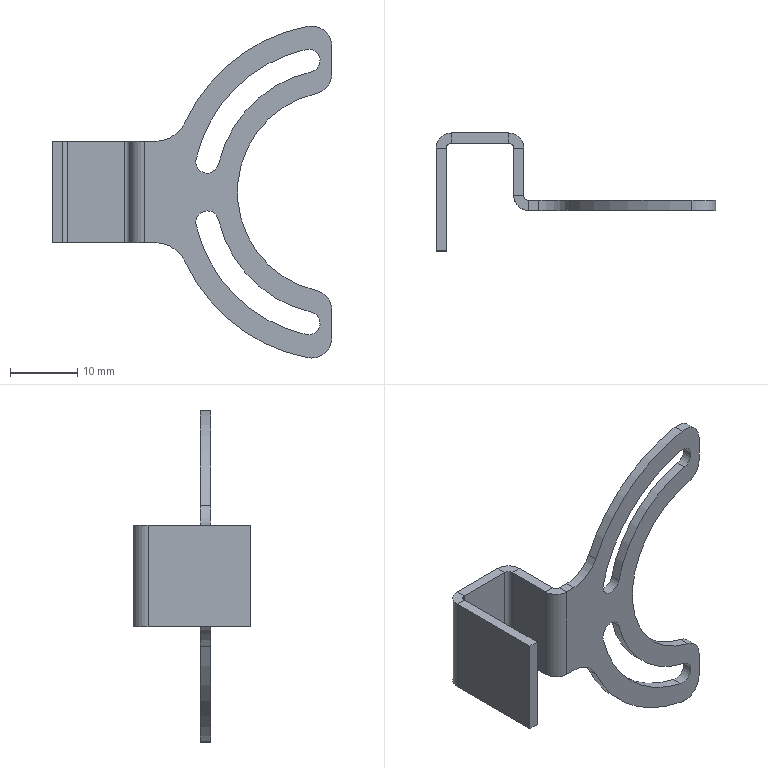Part | NX | features BREP 1 | 1 solid | 51 faces | box 41.5 x 17.5 x 49.267 mm | volume 1595 mm3 | cylinder 26 | plane 25 | commonest cylinder face diameters 3.4 x6 6 x5 1.473 x3 4.473 x3 10 x2 36.6 x2
STEP:
#1=CARTESIAN_POINT('',(27.,1.5,-24.633));
#2=VERTEX_POINT('',#1);
#3=CARTESIAN_POINT('',(26.455,1.5,-24.583));
#4=VERTEX_POINT('',#3);
#5=CARTESIAN_POINT('',(27.,1.5,-21.633));
#6=DIRECTION('',(0.,1.,0.));
#7=DIRECTION('',(0.,0.,-1.));
#8=AXIS2_PLACEMENT_3D('',#5,#6,#7);
#9=CIRCLE('',#8,3.);
#10=EDGE_CURVE('',#2,#4,#9,.T.);
#11=ORIENTED_EDGE('',*,*,#10,.F.);
#12=CARTESIAN_POINT('',(27.,0.,-24.633));
#13=VERTEX_POINT('',#12);
#14=CARTESIAN_POINT('',(27.,0.,-24.633));
#15=DIRECTION('',(0.,-1.,0.));
#16=VECTOR('',#15,1000.);
#17=LINE('',#14,#16);
#18=EDGE_CURVE('',#2,#13,#17,.T.);
#19=ORIENTED_EDGE('',*,*,#18,.T.);
#20=CARTESIAN_POINT('',(26.455,0.,-24.583));
#21=VERTEX_POINT('',#20);
#22=CARTESIAN_POINT('',(27.,0.,-21.633));
#23=DIRECTION('',(0.,-1.,0.));
#24=DIRECTION('',(0.,0.,-1.));
#25=AXIS2_PLACEMENT_3D('',#22,#23,#24);
#26=CIRCLE('',#25,3.);
#27=EDGE_CURVE('',#21,#13,#26,.T.);
#28=ORIENTED_EDGE('',*,*,#27,.F.);
#29=CARTESIAN_POINT('',(26.455,0.,-24.583));
#30=DIRECTION('',(0.,-1.,0.));
#31=VECTOR('',#30,1000.);
#32=LINE('',#29,#31);
#33=EDGE_CURVE('',#4,#21,#32,.T.);
#34=ORIENTED_EDGE('',*,*,#33,.F.);
#35=EDGE_LOOP('',(#11,#19,#28,#34));
#36=FACE_BOUND('',#35,.T.);
#37=CARTESIAN_POINT('',(27.,0.,-21.633));
#38=DIRECTION('',(0.,-1.,0.));
#39=DIRECTION('',(0.,0.,1.));
#40=AXIS2_PLACEMENT_3D('',#37,#38,#39);
#41=CYLINDRICAL_SURFACE('',#40,3.);
#42=ADVANCED_FACE('',(#36),#41,.T.);
#43=CARTESIAN_POINT('',(26.934,0.,17.843));
#44=VERTEX_POINT('',#43);
#45=CARTESIAN_POINT('',(26.556,0.,21.2));
#46=VERTEX_POINT('',#45);
#47=CARTESIAN_POINT('',(26.556,0.,19.5));
#48=DIRECTION('',(0.,-1.,0.));
#49=DIRECTION('',(0.,0.,-1.));
#50=AXIS2_PLACEMENT_3D('',#47,#48,#49);
#51=CIRCLE('',#50,1.7);
#52=EDGE_CURVE('',#44,#46,#51,.T.);
#53=ORIENTED_EDGE('',*,*,#52,.T.);
#54=CARTESIAN_POINT('',(26.556,1.5,21.2));
#55=VERTEX_POINT('',#54);
#56=CARTESIAN_POINT('',(26.556,-6.,21.2));
#57=DIRECTION('',(0.,1.,0.));
#58=VECTOR('',#57,1000.);
#59=LINE('',#56,#58);
#60=EDGE_CURVE('',#46,#55,#59,.T.);
#61=ORIENTED_EDGE('',*,*,#60,.T.);
#62=CARTESIAN_POINT('',(26.934,1.5,17.843));
#63=VERTEX_POINT('',#62);
#64=CARTESIAN_POINT('',(26.556,1.5,19.5));
#65=DIRECTION('',(0.,-1.,0.));
#66=DIRECTION('',(0.,0.,-1.));
#67=AXIS2_PLACEMENT_3D('',#64,#65,#66);
#68=CIRCLE('',#67,1.7);
#69=EDGE_CURVE('',#63,#55,#68,.T.);
#70=ORIENTED_EDGE('',*,*,#69,.F.);
#71=CARTESIAN_POINT('',(26.934,-6.,17.843));
#72=DIRECTION('',(0.,1.,0.));
#73=VECTOR('',#72,1000.);
#74=LINE('',#71,#73);
#75=EDGE_CURVE('',#44,#63,#74,.T.);
#76=ORIENTED_EDGE('',*,*,#75,.F.);
#77=EDGE_LOOP('',(#53,#61,#70,#76));
#78=FACE_BOUND('',#77,.T.);
#79=CARTESIAN_POINT('',(26.556,-6.,19.5));
#80=DIRECTION('',(0.,1.,0.));
#81=DIRECTION('',(0.,0.,-1.));
#82=AXIS2_PLACEMENT_3D('',#79,#80,#81);
#83=CYLINDRICAL_SURFACE('',#82,1.7);
#84=ADVANCED_FACE('',(#78),#83,.F.);
#85=CARTESIAN_POINT('',(13.169,0.,-4.117));
#86=VERTEX_POINT('',#85);
#87=CARTESIAN_POINT('',(11.513,0.,-2.8));
#88=VERTEX_POINT('',#87);
#89=CARTESIAN_POINT('',(11.513,0.,-4.5));
#90=DIRECTION('',(0.,-1.,0.));
#91=DIRECTION('',(0.,0.,-1.));
#92=AXIS2_PLACEMENT_3D('',#89,#90,#91);
#93=CIRCLE('',#92,1.7);
#94=EDGE_CURVE('',#86,#88,#93,.T.);
#95=ORIENTED_EDGE('',*,*,#94,.T.);
#96=CARTESIAN_POINT('',(11.513,1.5,-2.8));
#97=VERTEX_POINT('',#96);
#98=CARTESIAN_POINT('',(11.513,-6.,-2.8));
#99=DIRECTION('',(0.,1.,0.));
#100=VECTOR('',#99,1000.);
#101=LINE('',#98,#100);
#102=EDGE_CURVE('',#88,#97,#101,.T.);
#103=ORIENTED_EDGE('',*,*,#102,.T.);
#104=CARTESIAN_POINT('',(13.169,1.5,-4.117));
#105=VERTEX_POINT('',#104);
#106=CARTESIAN_POINT('',(11.513,1.5,-4.5));
#107=DIRECTION('',(0.,-1.,0.));
#108=DIRECTION('',(0.,0.,-1.));
#109=AXIS2_PLACEMENT_3D('',#106,#107,#108);
#110=CIRCLE('',#109,1.7);
#111=EDGE_CURVE('',#105,#97,#110,.T.);
#112=ORIENTED_EDGE('',*,*,#111,.F.);
#113=CARTESIAN_POINT('',(13.169,-6.,-4.117));
#114=DIRECTION('',(0.,1.,0.));
#115=VECTOR('',#114,1000.);
#116=LINE('',#113,#115);
#117=EDGE_CURVE('',#86,#105,#116,.T.);
#118=ORIENTED_EDGE('',*,*,#117,.F.);
#119=EDGE_LOOP('',(#95,#103,#112,#118));
#120=FACE_BOUND('',#119,.T.);
#121=CARTESIAN_POINT('',(11.513,-6.,-4.5));
#122=DIRECTION('',(0.,1.,0.));
#123=DIRECTION('',(0.,0.,-1.));
#124=AXIS2_PLACEMENT_3D('',#121,#122,#123);
#125=CYLINDRICAL_SURFACE('',#124,1.7);
#126=ADVANCED_FACE('',(#120),#125,.F.);
#127=CARTESIAN_POINT('',(26.178,0.,-21.157));
#128=VERTEX_POINT('',#127);
#129=CARTESIAN_POINT('',(26.934,0.,-17.843));
#130=VERTEX_POINT('',#129);
#131=CARTESIAN_POINT('',(26.556,0.,-19.5));
#132=DIRECTION('',(0.,-1.,0.));
#133=DIRECTION('',(0.,0.,-1.));
#134=AXIS2_PLACEMENT_3D('',#131,#132,#133);
#135=CIRCLE('',#134,1.7);
#136=EDGE_CURVE('',#128,#130,#135,.T.);
#137=ORIENTED_EDGE('',*,*,#136,.F.);
#138=CARTESIAN_POINT('',(9.856,0.,-4.883));
#139=VERTEX_POINT('',#138);
#140=CARTESIAN_POINT('',(31.,0.,0.));
#141=DIRECTION('',(0.,-1.,0.));
#142=DIRECTION('',(0.,0.,-1.));
#143=AXIS2_PLACEMENT_3D('',#140,#141,#142);
#144=CIRCLE('',#143,21.7);
#145=EDGE_CURVE('',#139,#128,#144,.T.);
#146=ORIENTED_EDGE('',*,*,#145,.F.);
#147=CARTESIAN_POINT('',(11.513,0.,-4.5));
#148=DIRECTION('',(0.,-1.,0.));
#149=DIRECTION('',(0.,0.,-1.));
#150=AXIS2_PLACEMENT_3D('',#147,#148,#149);
#151=CIRCLE('',#150,1.7);
#152=EDGE_CURVE('',#88,#139,#151,.T.);
#153=ORIENTED_EDGE('',*,*,#152,.F.);
#154=ORIENTED_EDGE('',*,*,#94,.F.);
#155=CARTESIAN_POINT('',(31.,0.,0.));
#156=DIRECTION('',(0.,1.,0.));
#157=DIRECTION('',(0.,0.,-1.));
#158=AXIS2_PLACEMENT_3D('',#155,#156,#157);
#159=CIRCLE('',#158,18.3);
#160=EDGE_CURVE('',#130,#86,#159,.T.);
#161=ORIENTED_EDGE('',*,*,#160,.F.);
#162=EDGE_LOOP('',(#137,#146,#153,#154,#161));
#163=FACE_BOUND('',#162,.T.);
#164=ORIENTED_EDGE('',*,*,#52,.F.);
#165=CARTESIAN_POINT('',(13.169,0.,4.117));
#166=VERTEX_POINT('',#165);
#167=CARTESIAN_POINT('',(31.,0.,0.));
#168=DIRECTION('',(0.,1.,0.));
#169=DIRECTION('',(0.,0.,-1.));
#170=AXIS2_PLACEMENT_3D('',#167,#168,#169);
#171=CIRCLE('',#170,18.3);
#172=EDGE_CURVE('',#166,#44,#171,.T.);
#173=ORIENTED_EDGE('',*,*,#172,.F.);
#174=CARTESIAN_POINT('',(9.856,0.,4.883));
#175=VERTEX_POINT('',#174);
#176=CARTESIAN_POINT('',(11.513,0.,4.5));
#177=DIRECTION('',(0.,-1.,0.));
#178=DIRECTION('',(0.,0.,-1.));
#179=AXIS2_PLACEMENT_3D('',#176,#177,#178);
#180=CIRCLE('',#179,1.7);
#181=EDGE_CURVE('',#175,#166,#180,.T.);
#182=ORIENTED_EDGE('',*,*,#181,.F.);
#183=CARTESIAN_POINT('',(26.178,0.,21.157));
#184=VERTEX_POINT('',#183);
#185=CARTESIAN_POINT('',(31.,0.,0.));
#186=DIRECTION('',(0.,-1.,0.));
#187=DIRECTION('',(0.,0.,-1.));
#188=AXIS2_PLACEMENT_3D('',#185,#186,#187);
#189=CIRCLE('',#188,21.7);
#190=EDGE_CURVE('',#184,#175,#189,.T.);
#191=ORIENTED_EDGE('',*,*,#190,.F.);
#192=CARTESIAN_POINT('',(26.556,0.,19.5));
#193=DIRECTION('',(0.,-1.,0.));
#194=DIRECTION('',(0.,0.,-1.));
#195=AXIS2_PLACEMENT_3D('',#192,#193,#194);
#196=CIRCLE('',#195,1.7);
#197=EDGE_CURVE('',#46,#184,#196,.T.);
#198=ORIENTED_EDGE('',*,*,#197,.F.);
#199=EDGE_LOOP('',(#164,#173,#182,#191,#198));
#200=FACE_BOUND('',#199,.T.);
#201=CARTESIAN_POINT('',(8.274,0.,-10.417));
#202=VERTEX_POINT('',#201);
#203=CARTESIAN_POINT('',(31.,0.,0.));
#204=DIRECTION('',(0.,1.,0.));
#205=DIRECTION('',(0.,0.,-1.));
#206=AXIS2_PLACEMENT_3D('',#203,#204,#205);
#207=CIRCLE('',#206,25.);
#208=EDGE_CURVE('',#21,#202,#207,.T.);
#209=ORIENTED_EDGE('',*,*,#208,.F.);
#210=ORIENTED_EDGE('',*,*,#27,.T.);
#211=CARTESIAN_POINT('',(30.,0.,-21.633));
#212=VERTEX_POINT('',#211);
#213=CARTESIAN_POINT('',(27.,0.,-21.633));
#214=DIRECTION('',(0.,-1.,0.));
#215=DIRECTION('',(0.,0.,-1.));
#216=AXIS2_PLACEMENT_3D('',#213,#214,#215);
#217=CIRCLE('',#216,3.);
#218=EDGE_CURVE('',#13,#212,#217,.T.);
#219=ORIENTED_EDGE('',*,*,#218,.T.);
#220=CARTESIAN_POINT('',(30.,0.,-17.55));
#221=VERTEX_POINT('',#220);
#222=CARTESIAN_POINT('',(30.,0.,25.));
#223=DIRECTION('',(0.,0.,-1.));
#224=VECTOR('',#223,1000.);
#225=LINE('',#222,#224);
#226=EDGE_CURVE('',#221,#212,#225,.T.);
#227=ORIENTED_EDGE('',*,*,#226,.F.);
#228=CARTESIAN_POINT('',(27.667,0.,-14.625));
#229=VERTEX_POINT('',#228);
#230=CARTESIAN_POINT('',(27.,0.,-17.55));
#231=DIRECTION('',(0.,-1.,0.));
#232=DIRECTION('',(0.,0.,-1.));
#233=AXIS2_PLACEMENT_3D('',#230,#231,#232);
#234=CIRCLE('',#233,3.);
#235=EDGE_CURVE('',#221,#229,#234,.T.);
#236=ORIENTED_EDGE('',*,*,#235,.T.);
#237=CARTESIAN_POINT('',(27.667,0.,14.625));
#238=VERTEX_POINT('',#237);
#239=CARTESIAN_POINT('',(31.,0.,0.));
#240=DIRECTION('',(0.,-1.,0.));
#241=DIRECTION('',(0.,0.,-1.));
#242=AXIS2_PLACEMENT_3D('',#239,#240,#241);
#243=CIRCLE('',#242,15.);
#244=EDGE_CURVE('',#238,#229,#243,.T.);
#245=ORIENTED_EDGE('',*,*,#244,.F.);
#246=CARTESIAN_POINT('',(30.,0.,17.55));
#247=VERTEX_POINT('',#246);
#248=CARTESIAN_POINT('',(27.,0.,17.55));
#249=DIRECTION('',(0.,-1.,0.));
#250=DIRECTION('',(0.,0.,-1.));
#251=AXIS2_PLACEMENT_3D('',#248,#249,#250);
#252=CIRCLE('',#251,3.);
#253=EDGE_CURVE('',#238,#247,#252,.T.);
#254=ORIENTED_EDGE('',*,*,#253,.T.);
#255=CARTESIAN_POINT('',(30.,0.,21.633));
#256=VERTEX_POINT('',#255);
#257=CARTESIAN_POINT('',(30.,0.,25.));
#258=DIRECTION('',(0.,0.,-1.));
#259=VECTOR('',#258,1000.);
#260=LINE('',#257,#259);
#261=EDGE_CURVE('',#256,#247,#260,.T.);
#262=ORIENTED_EDGE('',*,*,#261,.F.);
#263=CARTESIAN_POINT('',(26.455,0.,24.583));
#264=VERTEX_POINT('',#263);
#265=CARTESIAN_POINT('',(27.,0.,21.633));
#266=DIRECTION('',(0.,-1.,0.));
#267=DIRECTION('',(0.,0.,-1.));
#268=AXIS2_PLACEMENT_3D('',#265,#266,#267);
#269=CIRCLE('',#268,3.);
#270=EDGE_CURVE('',#256,#264,#269,.T.);
#271=ORIENTED_EDGE('',*,*,#270,.T.);
#272=CARTESIAN_POINT('',(8.274,0.,10.417));
#273=VERTEX_POINT('',#272);
#274=CARTESIAN_POINT('',(31.,0.,0.));
#275=DIRECTION('',(0.,1.,0.));
#276=DIRECTION('',(0.,0.,-1.));
#277=AXIS2_PLACEMENT_3D('',#274,#275,#276);
#278=CIRCLE('',#277,25.);
#279=EDGE_CURVE('',#273,#264,#278,.T.);
#280=ORIENTED_EDGE('',*,*,#279,.F.);
#281=CARTESIAN_POINT('',(3.728,0.,7.5));
#282=VERTEX_POINT('',#281);
#283=CARTESIAN_POINT('',(3.728,0.,12.5));
#284=DIRECTION('',(0.,1.,0.));
#285=DIRECTION('',(0.,0.,-1.));
#286=AXIS2_PLACEMENT_3D('',#283,#284,#285);
#287=CIRCLE('',#286,5.);
#288=EDGE_CURVE('',#273,#282,#287,.T.);
#289=ORIENTED_EDGE('',*,*,#288,.T.);
#290=CARTESIAN_POINT('',(2.237,0.,7.5));
#291=VERTEX_POINT('',#290);
#292=CARTESIAN_POINT('',(0.,0.,7.5));
#293=DIRECTION('',(1.,0.,0.));
#294=VECTOR('',#293,1000.);
#295=LINE('',#292,#294);
#296=EDGE_CURVE('',#291,#282,#295,.T.);
#297=ORIENTED_EDGE('',*,*,#296,.F.);
#298=CARTESIAN_POINT('',(2.237,0.,-7.5));
#299=VERTEX_POINT('',#298);
#300=CARTESIAN_POINT('',(2.237,0.,25.));
#301=DIRECTION('',(0.,0.,-1.));
#302=VECTOR('',#301,1000.);
#303=LINE('',#300,#302);
#304=EDGE_CURVE('',#291,#299,#303,.T.);
#305=ORIENTED_EDGE('',*,*,#304,.T.);
#306=CARTESIAN_POINT('',(3.728,0.,-7.5));
#307=VERTEX_POINT('',#306);
#308=CARTESIAN_POINT('',(0.,0.,-7.5));
#309=DIRECTION('',(-1.,0.,0.));
#310=VECTOR('',#309,1000.);
#311=LINE('',#308,#310);
#312=EDGE_CURVE('',#307,#299,#311,.T.);
#313=ORIENTED_EDGE('',*,*,#312,.F.);
#314=CARTESIAN_POINT('',(3.728,0.,-12.5));
#315=DIRECTION('',(0.,1.,0.));
#316=DIRECTION('',(0.,0.,-1.));
#317=AXIS2_PLACEMENT_3D('',#314,#315,#316);
#318=CIRCLE('',#317,5.);
#319=EDGE_CURVE('',#307,#202,#318,.T.);
#320=ORIENTED_EDGE('',*,*,#319,.T.);
#321=EDGE_LOOP('',(#209,#210,#219,#227,#236,#245,#254,#262,#271,#280,#289,#297,#305,#313,#320));
#322=FACE_BOUND('',#321,.T.);
#323=CARTESIAN_POINT('',(0.,0.,25.));
#324=DIRECTION('',(0.,-1.,0.));
#325=DIRECTION('',(0.,0.,1.));
#326=AXIS2_PLACEMENT_3D('',#323,#324,#325);
#327=PLANE('',#326);
#328=ADVANCED_FACE('',(#163,#200,#322),#327,.T.);
#329=CARTESIAN_POINT('',(9.856,1.5,-4.883));
#330=VERTEX_POINT('',#329);
#331=CARTESIAN_POINT('',(26.178,1.5,-21.157));
#332=VERTEX_POINT('',#331);
#333=CARTESIAN_POINT('',(31.,1.5,0.));
#334=DIRECTION('',(0.,-1.,0.));
#335=DIRECTION('',(0.,0.,-1.));
#336=AXIS2_PLACEMENT_3D('',#333,#334,#335);
#337=CIRCLE('',#336,21.7);
#338=EDGE_CURVE('',#330,#332,#337,.T.);
#339=ORIENTED_EDGE('',*,*,#338,.T.);
#340=CARTESIAN_POINT('',(26.934,1.5,-17.843));
#341=VERTEX_POINT('',#340);
#342=CARTESIAN_POINT('',(26.556,1.5,-19.5));
#343=DIRECTION('',(0.,-1.,0.));
#344=DIRECTION('',(0.,0.,-1.));
#345=AXIS2_PLACEMENT_3D('',#342,#343,#344);
#346=CIRCLE('',#345,1.7);
#347=EDGE_CURVE('',#332,#341,#346,.T.);
#348=ORIENTED_EDGE('',*,*,#347,.T.);
#349=CARTESIAN_POINT('',(31.,1.5,0.));
#350=DIRECTION('',(0.,1.,0.));
#351=DIRECTION('',(0.,0.,-1.));
#352=AXIS2_PLACEMENT_3D('',#349,#350,#351);
#353=CIRCLE('',#352,18.3);
#354=EDGE_CURVE('',#341,#105,#353,.T.);
#355=ORIENTED_EDGE('',*,*,#354,.T.);
#356=ORIENTED_EDGE('',*,*,#111,.T.);
#357=CARTESIAN_POINT('',(11.513,1.5,-4.5));
#358=DIRECTION('',(0.,-1.,0.));
#359=DIRECTION('',(0.,0.,-1.));
#360=AXIS2_PLACEMENT_3D('',#357,#358,#359);
#361=CIRCLE('',#360,1.7);
#362=EDGE_CURVE('',#97,#330,#361,.T.);
#363=ORIENTED_EDGE('',*,*,#362,.T.);
#364=EDGE_LOOP('',(#339,#348,#355,#356,#363));
#365=FACE_BOUND('',#364,.T.);
#366=CARTESIAN_POINT('',(13.169,1.5,4.117));
#367=VERTEX_POINT('',#366);
#368=CARTESIAN_POINT('',(31.,1.5,0.));
#369=DIRECTION('',(0.,1.,0.));
#370=DIRECTION('',(0.,0.,-1.));
#371=AXIS2_PLACEMENT_3D('',#368,#369,#370);
#372=CIRCLE('',#371,18.3);
#373=EDGE_CURVE('',#367,#63,#372,.T.);
#374=ORIENTED_EDGE('',*,*,#373,.T.);
#375=ORIENTED_EDGE('',*,*,#69,.T.);
#376=CARTESIAN_POINT('',(26.178,1.5,21.157));
#377=VERTEX_POINT('',#376);
#378=CARTESIAN_POINT('',(26.556,1.5,19.5));
#379=DIRECTION('',(0.,-1.,0.));
#380=DIRECTION('',(0.,0.,-1.));
#381=AXIS2_PLACEMENT_3D('',#378,#379,#380);
#382=CIRCLE('',#381,1.7);
#383=EDGE_CURVE('',#55,#377,#382,.T.);
#384=ORIENTED_EDGE('',*,*,#383,.T.);
#385=CARTESIAN_POINT('',(9.856,1.5,4.883));
#386=VERTEX_POINT('',#385);
#387=CARTESIAN_POINT('',(31.,1.5,0.));
#388=DIRECTION('',(0.,-1.,0.));
#389=DIRECTION('',(0.,0.,-1.));
#390=AXIS2_PLACEMENT_3D('',#387,#388,#389);
#391=CIRCLE('',#390,21.7);
#392=EDGE_CURVE('',#377,#386,#391,.T.);
#393=ORIENTED_EDGE('',*,*,#392,.T.);
#394=CARTESIAN_POINT('',(11.513,1.5,4.5));
#395=DIRECTION('',(0.,-1.,0.));
#396=DIRECTION('',(0.,0.,-1.));
#397=AXIS2_PLACEMENT_3D('',#394,#395,#396);
#398=CIRCLE('',#397,1.7);
#399=EDGE_CURVE('',#386,#367,#398,.T.);
#400=ORIENTED_EDGE('',*,*,#399,.T.);
#401=EDGE_LOOP('',(#374,#375,#384,#393,#400));
#402=FACE_BOUND('',#401,.T.);
#403=CARTESIAN_POINT('',(30.,1.5,-17.55));
#404=VERTEX_POINT('',#403);
#405=CARTESIAN_POINT('',(30.,1.5,-21.633));
#406=VERTEX_POINT('',#405);
#407=CARTESIAN_POINT('',(30.,1.5,25.));
#408=DIRECTION('',(0.,0.,-1.));
#409=VECTOR('',#408,1000.);
#410=LINE('',#407,#409);
#411=EDGE_CURVE('',#404,#406,#410,.T.);
#412=ORIENTED_EDGE('',*,*,#411,.T.);
#413=CARTESIAN_POINT('',(27.,1.5,-21.633));
#414=DIRECTION('',(0.,1.,0.));
#415=DIRECTION('',(0.,0.,-1.));
#416=AXIS2_PLACEMENT_3D('',#413,#414,#415);
#417=CIRCLE('',#416,3.);
#418=EDGE_CURVE('',#406,#2,#417,.T.);
#419=ORIENTED_EDGE('',*,*,#418,.T.);
#420=ORIENTED_EDGE('',*,*,#10,.T.);
#421=CARTESIAN_POINT('',(8.274,1.5,-10.417));
#422=VERTEX_POINT('',#421);
#423=CARTESIAN_POINT('',(31.,1.5,0.));
#424=DIRECTION('',(0.,1.,0.));
#425=DIRECTION('',(0.,0.,-1.));
#426=AXIS2_PLACEMENT_3D('',#423,#424,#425);
#427=CIRCLE('',#426,25.);
#428=EDGE_CURVE('',#4,#422,#427,.T.);
#429=ORIENTED_EDGE('',*,*,#428,.T.);
#430=CARTESIAN_POINT('',(3.728,1.5,-7.5));
#431=VERTEX_POINT('',#430);
#432=CARTESIAN_POINT('',(3.728,1.5,-12.5));
#433=DIRECTION('',(0.,-1.,0.));
#434=DIRECTION('',(0.,0.,-1.));
#435=AXIS2_PLACEMENT_3D('',#432,#433,#434);
#436=CIRCLE('',#435,5.);
#437=EDGE_CURVE('',#422,#431,#436,.T.);
#438=ORIENTED_EDGE('',*,*,#437,.T.);
#439=CARTESIAN_POINT('',(2.237,1.5,-7.5));
#440=VERTEX_POINT('',#439);
#441=CARTESIAN_POINT('',(0.,1.5,-7.5));
#442=DIRECTION('',(-1.,0.,0.));
#443=VECTOR('',#442,1000.);
#444=LINE('',#441,#443);
#445=EDGE_CURVE('',#431,#440,#444,.T.);
#446=ORIENTED_EDGE('',*,*,#445,.T.);
#447=CARTESIAN_POINT('',(2.237,1.5,7.5));
#448=VERTEX_POINT('',#447);
#449=CARTESIAN_POINT('',(2.237,1.5,25.));
#450=DIRECTION('',(0.,0.,-1.));
#451=VECTOR('',#450,1000.);
#452=LINE('',#449,#451);
#453=EDGE_CURVE('',#448,#440,#452,.T.);
#454=ORIENTED_EDGE('',*,*,#453,.F.);
#455=CARTESIAN_POINT('',(3.728,1.5,7.5));
#456=VERTEX_POINT('',#455);
#457=CARTESIAN_POINT('',(0.,1.5,7.5));
#458=DIRECTION('',(1.,0.,0.));
#459=VECTOR('',#458,1000.);
#460=LINE('',#457,#459);
#461=EDGE_CURVE('',#448,#456,#460,.T.);
#462=ORIENTED_EDGE('',*,*,#461,.T.);
#463=CARTESIAN_POINT('',(8.274,1.5,10.417));
#464=VERTEX_POINT('',#463);
#465=CARTESIAN_POINT('',(3.728,1.5,12.5));
#466=DIRECTION('',(0.,-1.,0.));
#467=DIRECTION('',(0.,0.,-1.));
#468=AXIS2_PLACEMENT_3D('',#465,#466,#467);
#469=CIRCLE('',#468,5.);
#470=EDGE_CURVE('',#456,#464,#469,.T.);
#471=ORIENTED_EDGE('',*,*,#470,.T.);
#472=CARTESIAN_POINT('',(26.455,1.5,24.583));
#473=VERTEX_POINT('',#472);
#474=CARTESIAN_POINT('',(31.,1.5,0.));
#475=DIRECTION('',(0.,1.,0.));
#476=DIRECTION('',(0.,0.,-1.));
#477=AXIS2_PLACEMENT_3D('',#474,#475,#476);
#478=CIRCLE('',#477,25.);
#479=EDGE_CURVE('',#464,#473,#478,.T.);
#480=ORIENTED_EDGE('',*,*,#479,.T.);
#481=CARTESIAN_POINT('',(30.,1.5,21.633));
#482=VERTEX_POINT('',#481);
#483=CARTESIAN_POINT('',(27.,1.5,21.633));
#484=DIRECTION('',(0.,1.,0.));
#485=DIRECTION('',(0.,0.,-1.));
#486=AXIS2_PLACEMENT_3D('',#483,#484,#485);
#487=CIRCLE('',#486,3.);
#488=EDGE_CURVE('',#473,#482,#487,.T.);
#489=ORIENTED_EDGE('',*,*,#488,.T.);
#490=CARTESIAN_POINT('',(30.,1.5,17.55));
#491=VERTEX_POINT('',#490);
#492=CARTESIAN_POINT('',(30.,1.5,25.));
#493=DIRECTION('',(0.,0.,-1.));
#494=VECTOR('',#493,1000.);
#495=LINE('',#492,#494);
#496=EDGE_CURVE('',#482,#491,#495,.T.);
#497=ORIENTED_EDGE('',*,*,#496,.T.);
#498=CARTESIAN_POINT('',(27.667,1.5,14.625));
#499=VERTEX_POINT('',#498);
#500=CARTESIAN_POINT('',(27.,1.5,17.55));
#501=DIRECTION('',(0.,1.,0.));
#502=DIRECTION('',(0.,0.,-1.));
#503=AXIS2_PLACEMENT_3D('',#500,#501,#502);
#504=CIRCLE('',#503,3.);
#505=EDGE_CURVE('',#491,#499,#504,.T.);
#506=ORIENTED_EDGE('',*,*,#505,.T.);
#507=CARTESIAN_POINT('',(27.667,1.5,-14.625));
#508=VERTEX_POINT('',#507);
#509=CARTESIAN_POINT('',(31.,1.5,0.));
#510=DIRECTION('',(0.,-1.,0.));
#511=DIRECTION('',(0.,0.,-1.));
#512=AXIS2_PLACEMENT_3D('',#509,#510,#511);
#513=CIRCLE('',#512,15.);
#514=EDGE_CURVE('',#499,#508,#513,.T.);
#515=ORIENTED_EDGE('',*,*,#514,.T.);
#516=CARTESIAN_POINT('',(27.,1.5,-17.55));
#517=DIRECTION('',(0.,1.,0.));
#518=DIRECTION('',(0.,0.,-1.));
#519=AXIS2_PLACEMENT_3D('',#516,#517,#518);
#520=CIRCLE('',#519,3.);
#521=EDGE_CURVE('',#508,#404,#520,.T.);
#522=ORIENTED_EDGE('',*,*,#521,.T.);
#523=EDGE_LOOP('',(#412,#419,#420,#429,#438,#446,#454,#462,#471,#480,#489,#497,#506,#515,#522));
#524=FACE_BOUND('',#523,.T.);
#525=CARTESIAN_POINT('',(0.,1.5,25.));
#526=DIRECTION('',(0.,-1.,0.));
#527=DIRECTION('',(0.,0.,1.));
#528=AXIS2_PLACEMENT_3D('',#525,#526,#527);
#529=PLANE('',#528);
#530=ADVANCED_FACE('',(#365,#402,#524),#529,.F.);
#531=CARTESIAN_POINT('',(-11.5,-6.,-7.5));
#532=VERTEX_POINT('',#531);
#533=CARTESIAN_POINT('',(-11.5,9.263,-7.5));
#534=VERTEX_POINT('',#533);
#535=CARTESIAN_POINT('',(-11.5,-6.,-7.5));
#536=DIRECTION('',(0.,1.,0.));
#537=VECTOR('',#536,1000.);
#538=LINE('',#535,#537);
#539=EDGE_CURVE('',#532,#534,#538,.T.);
#540=ORIENTED_EDGE('',*,*,#539,.F.);
#541=CARTESIAN_POINT('',(-11.5,-6.,7.5));
#542=VERTEX_POINT('',#541);
#543=CARTESIAN_POINT('',(-11.5,-6.,25.));
#544=DIRECTION('',(0.,0.,-1.));
#545=VECTOR('',#544,1000.);
#546=LINE('',#543,#545);
#547=EDGE_CURVE('',#542,#532,#546,.T.);
#548=ORIENTED_EDGE('',*,*,#547,.F.);
#549=CARTESIAN_POINT('',(-11.5,9.263,7.5));
#550=VERTEX_POINT('',#549);
#551=CARTESIAN_POINT('',(-11.5,10.,7.5));
#552=DIRECTION('',(0.,1.,0.));
#553=VECTOR('',#552,1000.);
#554=LINE('',#551,#553);
#555=EDGE_CURVE('',#542,#550,#554,.T.);
#556=ORIENTED_EDGE('',*,*,#555,.T.);
#557=CARTESIAN_POINT('',(-11.5,9.263,25.));
#558=DIRECTION('',(0.,0.,-1.));
#559=VECTOR('',#558,1000.);
#560=LINE('',#557,#559);
#561=EDGE_CURVE('',#550,#534,#560,.T.);
#562=ORIENTED_EDGE('',*,*,#561,.T.);
#563=EDGE_LOOP('',(#540,#548,#556,#562));
#564=FACE_BOUND('',#563,.T.);
#565=CARTESIAN_POINT('',(-11.5,10.,25.));
#566=DIRECTION('',(1.,0.,0.));
#567=DIRECTION('',(0.,0.,1.));
#568=AXIS2_PLACEMENT_3D('',#565,#566,#567);
#569=PLANE('',#568);
#570=ADVANCED_FACE('',(#564),#569,.F.);
#571=ORIENTED_EDGE('',*,*,#547,.T.);
#572=CARTESIAN_POINT('',(-10.,-6.,-7.5));
#573=VERTEX_POINT('',#572);
#574=CARTESIAN_POINT('',(-11.5,-6.,-7.5));
#575=DIRECTION('',(1.,0.,0.));
#576=VECTOR('',#575,1000.);
#577=LINE('',#574,#576);
#578=EDGE_CURVE('',#532,#573,#577,.T.);
#579=ORIENTED_EDGE('',*,*,#578,.T.);
#580=CARTESIAN_POINT('',(-10.,-6.,7.5));
#581=VERTEX_POINT('',#580);
#582=CARTESIAN_POINT('',(-10.,-6.,25.));
#583=DIRECTION('',(0.,0.,-1.));
#584=VECTOR('',#583,1000.);
#585=LINE('',#582,#584);
#586=EDGE_CURVE('',#581,#573,#585,.T.);
#587=ORIENTED_EDGE('',*,*,#586,.F.);
#588=CARTESIAN_POINT('',(-10.,-6.,7.5));
#589=DIRECTION('',(-1.,0.,0.));
#590=VECTOR('',#589,1000.);
#591=LINE('',#588,#590);
#592=EDGE_CURVE('',#581,#542,#591,.T.);
#593=ORIENTED_EDGE('',*,*,#592,.T.);
#594=EDGE_LOOP('',(#571,#579,#587,#593));
#595=FACE_BOUND('',#594,.T.);
#596=CARTESIAN_POINT('',(-10.,-6.,25.));
#597=DIRECTION('',(0.,-1.,0.));
#598=DIRECTION('',(0.,0.,1.));
#599=AXIS2_PLACEMENT_3D('',#596,#597,#598);
#600=PLANE('',#599);
#601=ADVANCED_FACE('',(#595),#600,.T.);
#602=ORIENTED_EDGE('',*,*,#586,.T.);
#603=CARTESIAN_POINT('',(-10.,9.263,-7.5));
#604=VERTEX_POINT('',#603);
#605=CARTESIAN_POINT('',(-10.,10.,-7.5));
#606=DIRECTION('',(0.,1.,0.));
#607=VECTOR('',#606,1000.);
#608=LINE('',#605,#607);
#609=EDGE_CURVE('',#573,#604,#608,.T.);
#610=ORIENTED_EDGE('',*,*,#609,.T.);
#611=CARTESIAN_POINT('',(-10.,9.263,7.5));
#612=VERTEX_POINT('',#611);
#613=CARTESIAN_POINT('',(-10.,9.263,25.));
#614=DIRECTION('',(0.,0.,-1.));
#615=VECTOR('',#614,1000.);
#616=LINE('',#613,#615);
#617=EDGE_CURVE('',#612,#604,#616,.T.);
#618=ORIENTED_EDGE('',*,*,#617,.F.);
#619=CARTESIAN_POINT('',(-10.,10.,7.5));
#620=DIRECTION('',(0.,1.,0.));
#621=VECTOR('',#620,1000.);
#622=LINE('',#619,#621);
#623=EDGE_CURVE('',#581,#612,#622,.T.);
#624=ORIENTED_EDGE('',*,*,#623,.F.);
#625=EDGE_LOOP('',(#602,#610,#618,#624));
#626=FACE_BOUND('',#625,.T.);
#627=CARTESIAN_POINT('',(-10.,10.,25.));
#628=DIRECTION('',(1.,0.,0.));
#629=DIRECTION('',(0.,0.,1.));
#630=AXIS2_PLACEMENT_3D('',#627,#628,#629);
#631=PLANE('',#630);
#632=ADVANCED_FACE('',(#626),#631,.T.);
#633=ORIENTED_EDGE('',*,*,#617,.T.);
#634=CARTESIAN_POINT('',(-9.263,10.,-7.5));
#635=VERTEX_POINT('',#634);
#636=CARTESIAN_POINT('',(-9.263,9.263,-7.5));
#637=DIRECTION('',(0.,0.,1.));
#638=DIRECTION('',(-1.,0.,0.));
#639=AXIS2_PLACEMENT_3D('',#636,#637,#638);
#640=CIRCLE('',#639,0.7366);
#641=EDGE_CURVE('',#635,#604,#640,.T.);
#642=ORIENTED_EDGE('',*,*,#641,.F.);
#643=CARTESIAN_POINT('',(-9.263,10.,7.5));
#644=VERTEX_POINT('',#643);
#645=CARTESIAN_POINT('',(-9.263,10.,25.));
#646=DIRECTION('',(0.,0.,-1.));
#647=VECTOR('',#646,1000.);
#648=LINE('',#645,#647);
#649=EDGE_CURVE('',#644,#635,#648,.T.);
#650=ORIENTED_EDGE('',*,*,#649,.F.);
#651=CARTESIAN_POINT('',(-9.263,9.263,7.5));
#652=DIRECTION('',(0.,0.,-1.));
#653=DIRECTION('',(-1.,0.,0.));
#654=AXIS2_PLACEMENT_3D('',#651,#652,#653);
#655=CIRCLE('',#654,0.7366);
#656=EDGE_CURVE('',#612,#644,#655,.T.);
#657=ORIENTED_EDGE('',*,*,#656,.F.);
#658=EDGE_LOOP('',(#633,#642,#650,#657));
#659=FACE_BOUND('',#658,.T.);
#660=CARTESIAN_POINT('',(-9.263,9.263,25.));
#661=DIRECTION('',(0.,0.,-1.));
#662=DIRECTION('',(1.,0.,0.));
#663=AXIS2_PLACEMENT_3D('',#660,#661,#662);
#664=CYLINDRICAL_SURFACE('',#663,0.7366);
#665=ADVANCED_FACE('',(#659),#664,.F.);
#666=ORIENTED_EDGE('',*,*,#649,.T.);
#667=CARTESIAN_POINT('',(-0.7366,10.,-7.5));
#668=VERTEX_POINT('',#667);
#669=CARTESIAN_POINT('',(0.,10.,-7.5));
#670=DIRECTION('',(-1.,0.,0.));
#671=VECTOR('',#670,1000.);
#672=LINE('',#669,#671);
#673=EDGE_CURVE('',#668,#635,#672,.T.);
#674=ORIENTED_EDGE('',*,*,#673,.F.);
#675=CARTESIAN_POINT('',(-0.7366,10.,7.5));
#676=VERTEX_POINT('',#675);
#677=CARTESIAN_POINT('',(-0.7366,10.,25.));
#678=DIRECTION('',(0.,0.,-1.));
#679=VECTOR('',#678,1000.);
#680=LINE('',#677,#679);
#681=EDGE_CURVE('',#676,#668,#680,.T.);
#682=ORIENTED_EDGE('',*,*,#681,.F.);
#683=CARTESIAN_POINT('',(0.,10.,7.5));
#684=DIRECTION('',(1.,0.,0.));
#685=VECTOR('',#684,1000.);
#686=LINE('',#683,#685);
#687=EDGE_CURVE('',#644,#676,#686,.T.);
#688=ORIENTED_EDGE('',*,*,#687,.F.);
#689=EDGE_LOOP('',(#666,#674,#682,#688));
#690=FACE_BOUND('',#689,.T.);
#691=CARTESIAN_POINT('',(0.,10.,25.));
#692=DIRECTION('',(0.,-1.,0.));
#693=DIRECTION('',(-1.,0.,0.));
#694=AXIS2_PLACEMENT_3D('',#691,#692,#693);
#695=PLANE('',#694);
#696=ADVANCED_FACE('',(#690),#695,.T.);
#697=ORIENTED_EDGE('',*,*,#681,.T.);
#698=CARTESIAN_POINT('',(0.,9.263,-7.5));
#699=VERTEX_POINT('',#698);
#700=CARTESIAN_POINT('',(-0.7366,9.263,-7.5));
#701=DIRECTION('',(0.,0.,1.));
#702=DIRECTION('',(-1.,0.,0.));
#703=AXIS2_PLACEMENT_3D('',#700,#701,#702);
#704=CIRCLE('',#703,0.7366);
#705=EDGE_CURVE('',#699,#668,#704,.T.);
#706=ORIENTED_EDGE('',*,*,#705,.F.);
#707=CARTESIAN_POINT('',(0.,9.263,7.5));
#708=VERTEX_POINT('',#707);
#709=CARTESIAN_POINT('',(0.,9.263,25.));
#710=DIRECTION('',(0.,0.,-1.));
#711=VECTOR('',#710,1000.);
#712=LINE('',#709,#711);
#713=EDGE_CURVE('',#708,#699,#712,.T.);
#714=ORIENTED_EDGE('',*,*,#713,.F.);
#715=CARTESIAN_POINT('',(-0.7366,9.263,7.5));
#716=DIRECTION('',(0.,0.,-1.));
#717=DIRECTION('',(-1.,0.,0.));
#718=AXIS2_PLACEMENT_3D('',#715,#716,#717);
#719=CIRCLE('',#718,0.7366);
#720=EDGE_CURVE('',#676,#708,#719,.T.);
#721=ORIENTED_EDGE('',*,*,#720,.F.);
#722=EDGE_LOOP('',(#697,#706,#714,#721));
#723=FACE_BOUND('',#722,.T.);
#724=CARTESIAN_POINT('',(-0.7366,9.263,25.));
#725=DIRECTION('',(0.,0.,-1.));
#726=DIRECTION('',(1.,0.,0.));
#727=AXIS2_PLACEMENT_3D('',#724,#725,#726);
#728=CYLINDRICAL_SURFACE('',#727,0.7366);
#729=ADVANCED_FACE('',(#723),#728,.F.);
#730=ORIENTED_EDGE('',*,*,#713,.T.);
#731=CARTESIAN_POINT('',(0.,2.237,-7.5));
#732=VERTEX_POINT('',#731);
#733=CARTESIAN_POINT('',(0.,0.,-7.5));
#734=DIRECTION('',(0.,1.,0.));
#735=VECTOR('',#734,1000.);
#736=LINE('',#733,#735);
#737=EDGE_CURVE('',#732,#699,#736,.T.);
#738=ORIENTED_EDGE('',*,*,#737,.F.);
#739=CARTESIAN_POINT('',(0.,2.237,7.5));
#740=VERTEX_POINT('',#739);
#741=CARTESIAN_POINT('',(0.,2.237,25.));
#742=DIRECTION('',(0.,0.,-1.));
#743=VECTOR('',#742,1000.);
#744=LINE('',#741,#743);
#745=EDGE_CURVE('',#740,#732,#744,.T.);
#746=ORIENTED_EDGE('',*,*,#745,.F.);
#747=CARTESIAN_POINT('',(0.,0.,7.5));
#748=DIRECTION('',(0.,-1.,0.));
#749=VECTOR('',#748,1000.);
#750=LINE('',#747,#749);
#751=EDGE_CURVE('',#708,#740,#750,.T.);
#752=ORIENTED_EDGE('',*,*,#751,.F.);
#753=EDGE_LOOP('',(#730,#738,#746,#752));
#754=FACE_BOUND('',#753,.T.);
#755=CARTESIAN_POINT('',(0.,0.,25.));
#756=DIRECTION('',(-1.,0.,0.));
#757=DIRECTION('',(0.,0.,-1.));
#758=AXIS2_PLACEMENT_3D('',#755,#756,#757);
#759=PLANE('',#758);
#760=ADVANCED_FACE('',(#754),#759,.T.);
#761=ORIENTED_EDGE('',*,*,#745,.T.);
#762=CARTESIAN_POINT('',(2.237,2.237,-7.5));
#763=DIRECTION('',(0.,0.,-1.));
#764=DIRECTION('',(-1.,0.,0.));
#765=AXIS2_PLACEMENT_3D('',#762,#763,#764);
#766=CIRCLE('',#765,2.237);
#767=EDGE_CURVE('',#299,#732,#766,.T.);
#768=ORIENTED_EDGE('',*,*,#767,.F.);
#769=ORIENTED_EDGE('',*,*,#304,.F.);
#770=CARTESIAN_POINT('',(2.237,2.237,7.5));
#771=DIRECTION('',(0.,0.,1.));
#772=DIRECTION('',(-1.,0.,0.));
#773=AXIS2_PLACEMENT_3D('',#770,#771,#772);
#774=CIRCLE('',#773,2.237);
#775=EDGE_CURVE('',#740,#291,#774,.T.);
#776=ORIENTED_EDGE('',*,*,#775,.F.);
#777=EDGE_LOOP('',(#761,#768,#769,#776));
#778=FACE_BOUND('',#777,.T.);
#779=CARTESIAN_POINT('',(2.237,2.237,25.));
#780=DIRECTION('',(0.,0.,-1.));
#781=DIRECTION('',(1.,0.,0.));
#782=AXIS2_PLACEMENT_3D('',#779,#780,#781);
#783=CYLINDRICAL_SURFACE('',#782,2.237);
#784=ADVANCED_FACE('',(#778),#783,.T.);
#785=CARTESIAN_POINT('',(1.5,2.237,-7.5));
#786=VERTEX_POINT('',#785);
#787=CARTESIAN_POINT('',(2.237,2.237,-7.5));
#788=DIRECTION('',(0.,0.,-1.));
#789=DIRECTION('',(1.,0.,0.));
#790=AXIS2_PLACEMENT_3D('',#787,#788,#789);
#791=CIRCLE('',#790,0.7366);
#792=EDGE_CURVE('',#440,#786,#791,.T.);
#793=ORIENTED_EDGE('',*,*,#792,.T.);
#794=CARTESIAN_POINT('',(1.5,2.237,7.5));
#795=VERTEX_POINT('',#794);
#796=CARTESIAN_POINT('',(1.5,2.237,25.));
#797=DIRECTION('',(0.,0.,-1.));
#798=VECTOR('',#797,1000.);
#799=LINE('',#796,#798);
#800=EDGE_CURVE('',#795,#786,#799,.T.);
#801=ORIENTED_EDGE('',*,*,#800,.F.);
#802=CARTESIAN_POINT('',(2.237,2.237,7.5));
#803=DIRECTION('',(0.,0.,1.));
#804=DIRECTION('',(-1.,0.,0.));
#805=AXIS2_PLACEMENT_3D('',#802,#803,#804);
#806=CIRCLE('',#805,0.7366);
#807=EDGE_CURVE('',#795,#448,#806,.T.);
#808=ORIENTED_EDGE('',*,*,#807,.T.);
#809=ORIENTED_EDGE('',*,*,#453,.T.);
#810=EDGE_LOOP('',(#793,#801,#808,#809));
#811=FACE_BOUND('',#810,.T.);
#812=CARTESIAN_POINT('',(2.237,2.237,25.));
#813=DIRECTION('',(0.,0.,-1.));
#814=DIRECTION('',(1.,0.,0.));
#815=AXIS2_PLACEMENT_3D('',#812,#813,#814);
#816=CYLINDRICAL_SURFACE('',#815,0.7366);
#817=ADVANCED_FACE('',(#811),#816,.F.);
#818=CARTESIAN_POINT('',(1.5,9.263,-7.5));
#819=VERTEX_POINT('',#818);
#820=CARTESIAN_POINT('',(1.5,0.,-7.5));
#821=DIRECTION('',(0.,1.,0.));
#822=VECTOR('',#821,1000.);
#823=LINE('',#820,#822);
#824=EDGE_CURVE('',#786,#819,#823,.T.);
#825=ORIENTED_EDGE('',*,*,#824,.T.);
#826=CARTESIAN_POINT('',(1.5,9.263,7.5));
#827=VERTEX_POINT('',#826);
#828=CARTESIAN_POINT('',(1.5,9.263,25.));
#829=DIRECTION('',(0.,0.,-1.));
#830=VECTOR('',#829,1000.);
#831=LINE('',#828,#830);
#832=EDGE_CURVE('',#827,#819,#831,.T.);
#833=ORIENTED_EDGE('',*,*,#832,.F.);
#834=CARTESIAN_POINT('',(1.5,0.,7.5));
#835=DIRECTION('',(0.,-1.,0.));
#836=VECTOR('',#835,1000.);
#837=LINE('',#834,#836);
#838=EDGE_CURVE('',#827,#795,#837,.T.);
#839=ORIENTED_EDGE('',*,*,#838,.T.);
#840=ORIENTED_EDGE('',*,*,#800,.T.);
#841=EDGE_LOOP('',(#825,#833,#839,#840));
#842=FACE_BOUND('',#841,.T.);
#843=CARTESIAN_POINT('',(1.5,0.,25.));
#844=DIRECTION('',(-1.,0.,0.));
#845=DIRECTION('',(0.,0.,-1.));
#846=AXIS2_PLACEMENT_3D('',#843,#844,#845);
#847=PLANE('',#846);
#848=ADVANCED_FACE('',(#842),#847,.F.);
#849=CARTESIAN_POINT('',(-0.7366,11.5,-7.5));
#850=VERTEX_POINT('',#849);
#851=CARTESIAN_POINT('',(-0.7366,9.263,-7.5));
#852=DIRECTION('',(0.,0.,1.));
#853=DIRECTION('',(1.,0.,0.));
#854=AXIS2_PLACEMENT_3D('',#851,#852,#853);
#855=CIRCLE('',#854,2.237);
#856=EDGE_CURVE('',#819,#850,#855,.T.);
#857=ORIENTED_EDGE('',*,*,#856,.T.);
#858=CARTESIAN_POINT('',(-0.7366,11.5,7.5));
#859=VERTEX_POINT('',#858);
#860=CARTESIAN_POINT('',(-0.7366,11.5,25.));
#861=DIRECTION('',(0.,0.,-1.));
#862=VECTOR('',#861,1000.);
#863=LINE('',#860,#862);
#864=EDGE_CURVE('',#859,#850,#863,.T.);
#865=ORIENTED_EDGE('',*,*,#864,.F.);
#866=CARTESIAN_POINT('',(-0.7366,9.263,7.5));
#867=DIRECTION('',(0.,0.,-1.));
#868=DIRECTION('',(-1.,0.,0.));
#869=AXIS2_PLACEMENT_3D('',#866,#867,#868);
#870=CIRCLE('',#869,2.237);
#871=EDGE_CURVE('',#859,#827,#870,.T.);
#872=ORIENTED_EDGE('',*,*,#871,.T.);
#873=ORIENTED_EDGE('',*,*,#832,.T.);
#874=EDGE_LOOP('',(#857,#865,#872,#873));
#875=FACE_BOUND('',#874,.T.);
#876=CARTESIAN_POINT('',(-0.7366,9.263,25.));
#877=DIRECTION('',(0.,0.,-1.));
#878=DIRECTION('',(1.,0.,0.));
#879=AXIS2_PLACEMENT_3D('',#876,#877,#878);
#880=CYLINDRICAL_SURFACE('',#879,2.237);
#881=ADVANCED_FACE('',(#875),#880,.T.);
#882=CARTESIAN_POINT('',(-9.263,11.5,-7.5));
#883=VERTEX_POINT('',#882);
#884=CARTESIAN_POINT('',(0.,11.5,-7.5));
#885=DIRECTION('',(-1.,0.,0.));
#886=VECTOR('',#885,1000.);
#887=LINE('',#884,#886);
#888=EDGE_CURVE('',#850,#883,#887,.T.);
#889=ORIENTED_EDGE('',*,*,#888,.T.);
#890=CARTESIAN_POINT('',(-9.263,11.5,7.5));
#891=VERTEX_POINT('',#890);
#892=CARTESIAN_POINT('',(-9.263,11.5,25.));
#893=DIRECTION('',(0.,0.,-1.));
#894=VECTOR('',#893,1000.);
#895=LINE('',#892,#894);
#896=EDGE_CURVE('',#891,#883,#895,.T.);
#897=ORIENTED_EDGE('',*,*,#896,.F.);
#898=CARTESIAN_POINT('',(0.,11.5,7.5));
#899=DIRECTION('',(1.,0.,0.));
#900=VECTOR('',#899,1000.);
#901=LINE('',#898,#900);
#902=EDGE_CURVE('',#891,#859,#901,.T.);
#903=ORIENTED_EDGE('',*,*,#902,.T.);
#904=ORIENTED_EDGE('',*,*,#864,.T.);
#905=EDGE_LOOP('',(#889,#897,#903,#904));
#906=FACE_BOUND('',#905,.T.);
#907=CARTESIAN_POINT('',(0.,11.5,25.));
#908=DIRECTION('',(0.,-1.,0.));
#909=DIRECTION('',(-1.,0.,0.));
#910=AXIS2_PLACEMENT_3D('',#907,#908,#909);
#911=PLANE('',#910);
#912=ADVANCED_FACE('',(#906),#911,.F.);
#913=CARTESIAN_POINT('',(-9.263,9.263,-7.5));
#914=DIRECTION('',(0.,0.,1.));
#915=DIRECTION('',(1.,0.,0.));
#916=AXIS2_PLACEMENT_3D('',#913,#914,#915);
#917=CIRCLE('',#916,2.237);
#918=EDGE_CURVE('',#883,#534,#917,.T.);
#919=ORIENTED_EDGE('',*,*,#918,.T.);
#920=ORIENTED_EDGE('',*,*,#561,.F.);
#921=CARTESIAN_POINT('',(-9.263,9.263,7.5));
#922=DIRECTION('',(0.,0.,-1.));
#923=DIRECTION('',(-1.,0.,0.));
#924=AXIS2_PLACEMENT_3D('',#921,#922,#923);
#925=CIRCLE('',#924,2.237);
#926=EDGE_CURVE('',#550,#891,#925,.T.);
#927=ORIENTED_EDGE('',*,*,#926,.T.);
#928=ORIENTED_EDGE('',*,*,#896,.T.);
#929=EDGE_LOOP('',(#919,#920,#927,#928));
#930=FACE_BOUND('',#929,.T.);
#931=CARTESIAN_POINT('',(-9.263,9.263,25.));
#932=DIRECTION('',(0.,0.,-1.));
#933=DIRECTION('',(1.,0.,0.));
#934=AXIS2_PLACEMENT_3D('',#931,#932,#933);
#935=CYLINDRICAL_SURFACE('',#934,2.237);
#936=ADVANCED_FACE('',(#930),#935,.T.);
#937=ORIENTED_EDGE('',*,*,#226,.T.);
#938=CARTESIAN_POINT('',(30.,1.5,-21.633));
#939=DIRECTION('',(0.,1.,0.));
#940=VECTOR('',#939,1000.);
#941=LINE('',#938,#940);
#942=EDGE_CURVE('',#212,#406,#941,.T.);
#943=ORIENTED_EDGE('',*,*,#942,.T.);
#944=ORIENTED_EDGE('',*,*,#411,.F.);
#945=CARTESIAN_POINT('',(30.,1.5,-17.55));
#946=DIRECTION('',(0.,-1.,0.));
#947=VECTOR('',#946,1000.);
#948=LINE('',#945,#947);
#949=EDGE_CURVE('',#404,#221,#948,.T.);
#950=ORIENTED_EDGE('',*,*,#949,.T.);
#951=EDGE_LOOP('',(#937,#943,#944,#950));
#952=FACE_BOUND('',#951,.T.);
#953=CARTESIAN_POINT('',(30.,1.5,25.));
#954=DIRECTION('',(1.,0.,0.));
#955=DIRECTION('',(0.,0.,1.));
#956=AXIS2_PLACEMENT_3D('',#953,#954,#955);
#957=PLANE('',#956);
#958=ADVANCED_FACE('',(#952),#957,.T.);
#959=ORIENTED_EDGE('',*,*,#261,.T.);
#960=CARTESIAN_POINT('',(30.,1.5,17.55));
#961=DIRECTION('',(0.,1.,0.));
#962=VECTOR('',#961,1000.);
#963=LINE('',#960,#962);
#964=EDGE_CURVE('',#247,#491,#963,.T.);
#965=ORIENTED_EDGE('',*,*,#964,.T.);
#966=ORIENTED_EDGE('',*,*,#496,.F.);
#967=CARTESIAN_POINT('',(30.,1.5,21.633));
#968=DIRECTION('',(0.,-1.,0.));
#969=VECTOR('',#968,1000.);
#970=LINE('',#967,#969);
#971=EDGE_CURVE('',#482,#256,#970,.T.);
#972=ORIENTED_EDGE('',*,*,#971,.T.);
#973=EDGE_LOOP('',(#959,#965,#966,#972));
#974=FACE_BOUND('',#973,.T.);
#975=CARTESIAN_POINT('',(30.,1.5,25.));
#976=DIRECTION('',(1.,0.,0.));
#977=DIRECTION('',(0.,0.,1.));
#978=AXIS2_PLACEMENT_3D('',#975,#976,#977);
#979=PLANE('',#978);
#980=ADVANCED_FACE('',(#974),#979,.T.);
#981=ORIENTED_EDGE('',*,*,#244,.T.);
#982=CARTESIAN_POINT('',(27.667,0.,-14.625));
#983=DIRECTION('',(0.,1.,0.));
#984=VECTOR('',#983,1000.);
#985=LINE('',#982,#984);
#986=EDGE_CURVE('',#229,#508,#985,.T.);
#987=ORIENTED_EDGE('',*,*,#986,.T.);
#988=ORIENTED_EDGE('',*,*,#514,.F.);
#989=CARTESIAN_POINT('',(27.667,0.,14.625));
#990=DIRECTION('',(0.,-1.,0.));
#991=VECTOR('',#990,1000.);
#992=LINE('',#989,#991);
#993=EDGE_CURVE('',#499,#238,#992,.T.);
#994=ORIENTED_EDGE('',*,*,#993,.T.);
#995=EDGE_LOOP('',(#981,#987,#988,#994));
#996=FACE_BOUND('',#995,.T.);
#997=CARTESIAN_POINT('',(31.,0.,0.));
#998=DIRECTION('',(0.,-1.,0.));
#999=DIRECTION('',(0.,0.,1.));
#1000=AXIS2_PLACEMENT_3D('',#997,#998,#999);
#1001=CYLINDRICAL_SURFACE('',#1000,15.);
#1002=ADVANCED_FACE('',(#996),#1001,.F.);
#1003=ORIENTED_EDGE('',*,*,#136,.T.);
#1004=CARTESIAN_POINT('',(26.934,-6.,-17.843));
#1005=DIRECTION('',(0.,1.,0.));
#1006=VECTOR('',#1005,1000.);
#1007=LINE('',#1004,#1006);
#1008=EDGE_CURVE('',#130,#341,#1007,.T.);
#1009=ORIENTED_EDGE('',*,*,#1008,.T.);
#1010=ORIENTED_EDGE('',*,*,#347,.F.);
#1011=CARTESIAN_POINT('',(26.178,-6.,-21.157));
#1012=DIRECTION('',(0.,1.,0.));
#1013=VECTOR('',#1012,1000.);
#1014=LINE('',#1011,#1013);
#1015=EDGE_CURVE('',#128,#332,#1014,.T.);
#1016=ORIENTED_EDGE('',*,*,#1015,.F.);
#1017=EDGE_LOOP('',(#1003,#1009,#1010,#1016));
#1018=FACE_BOUND('',#1017,.T.);
#1019=CARTESIAN_POINT('',(26.556,-6.,-19.5));
#1020=DIRECTION('',(0.,1.,0.));
#1021=DIRECTION('',(0.,0.,-1.));
#1022=AXIS2_PLACEMENT_3D('',#1019,#1020,#1021);
#1023=CYLINDRICAL_SURFACE('',#1022,1.7);
#1024=ADVANCED_FACE('',(#1018),#1023,.F.);
#1025=ORIENTED_EDGE('',*,*,#160,.T.);
#1026=ORIENTED_EDGE('',*,*,#117,.T.);
#1027=ORIENTED_EDGE('',*,*,#354,.F.);
#1028=ORIENTED_EDGE('',*,*,#1008,.F.);
#1029=EDGE_LOOP('',(#1025,#1026,#1027,#1028));
#1030=FACE_BOUND('',#1029,.T.);
#1031=CARTESIAN_POINT('',(31.,-6.,0.));
#1032=DIRECTION('',(0.,1.,0.));
#1033=DIRECTION('',(0.,0.,-1.));
#1034=AXIS2_PLACEMENT_3D('',#1031,#1032,#1033);
#1035=CYLINDRICAL_SURFACE('',#1034,18.3);
#1036=ADVANCED_FACE('',(#1030),#1035,.T.);
#1037=ORIENTED_EDGE('',*,*,#102,.F.);
#1038=ORIENTED_EDGE('',*,*,#152,.T.);
#1039=CARTESIAN_POINT('',(9.856,-6.,-4.883));
#1040=DIRECTION('',(0.,1.,0.));
#1041=VECTOR('',#1040,1000.);
#1042=LINE('',#1039,#1041);
#1043=EDGE_CURVE('',#139,#330,#1042,.T.);
#1044=ORIENTED_EDGE('',*,*,#1043,.T.);
#1045=ORIENTED_EDGE('',*,*,#362,.F.);
#1046=EDGE_LOOP('',(#1037,#1038,#1044,#1045));
#1047=FACE_BOUND('',#1046,.T.);
#1048=CARTESIAN_POINT('',(11.513,-6.,-4.5));
#1049=DIRECTION('',(0.,1.,0.));
#1050=DIRECTION('',(0.,0.,-1.));
#1051=AXIS2_PLACEMENT_3D('',#1048,#1049,#1050);
#1052=CYLINDRICAL_SURFACE('',#1051,1.7);
#1053=ADVANCED_FACE('',(#1047),#1052,.F.);
#1054=ORIENTED_EDGE('',*,*,#145,.T.);
#1055=ORIENTED_EDGE('',*,*,#1015,.T.);
#1056=ORIENTED_EDGE('',*,*,#338,.F.);
#1057=ORIENTED_EDGE('',*,*,#1043,.F.);
#1058=EDGE_LOOP('',(#1054,#1055,#1056,#1057));
#1059=FACE_BOUND('',#1058,.T.);
#1060=CARTESIAN_POINT('',(31.,-6.,0.));
#1061=DIRECTION('',(0.,1.,0.));
#1062=DIRECTION('',(0.,0.,-1.));
#1063=AXIS2_PLACEMENT_3D('',#1060,#1061,#1062);
#1064=CYLINDRICAL_SURFACE('',#1063,21.7);
#1065=ADVANCED_FACE('',(#1059),#1064,.F.);
#1066=ORIENTED_EDGE('',*,*,#60,.F.);
#1067=ORIENTED_EDGE('',*,*,#197,.T.);
#1068=CARTESIAN_POINT('',(26.178,-6.,21.157));
#1069=DIRECTION('',(0.,1.,0.));
#1070=VECTOR('',#1069,1000.);
#1071=LINE('',#1068,#1070);
#1072=EDGE_CURVE('',#184,#377,#1071,.T.);
#1073=ORIENTED_EDGE('',*,*,#1072,.T.);
#1074=ORIENTED_EDGE('',*,*,#383,.F.);
#1075=EDGE_LOOP('',(#1066,#1067,#1073,#1074));
#1076=FACE_BOUND('',#1075,.T.);
#1077=CARTESIAN_POINT('',(26.556,-6.,19.5));
#1078=DIRECTION('',(0.,1.,0.));
#1079=DIRECTION('',(0.,0.,-1.));
#1080=AXIS2_PLACEMENT_3D('',#1077,#1078,#1079);
#1081=CYLINDRICAL_SURFACE('',#1080,1.7);
#1082=ADVANCED_FACE('',(#1076),#1081,.F.);
#1083=ORIENTED_EDGE('',*,*,#190,.T.);
#1084=CARTESIAN_POINT('',(9.856,-6.,4.883));
#1085=DIRECTION('',(0.,1.,0.));
#1086=VECTOR('',#1085,1000.);
#1087=LINE('',#1084,#1086);
#1088=EDGE_CURVE('',#175,#386,#1087,.T.);
#1089=ORIENTED_EDGE('',*,*,#1088,.T.);
#1090=ORIENTED_EDGE('',*,*,#392,.F.);
#1091=ORIENTED_EDGE('',*,*,#1072,.F.);
#1092=EDGE_LOOP('',(#1083,#1089,#1090,#1091));
#1093=FACE_BOUND('',#1092,.T.);
#1094=CARTESIAN_POINT('',(31.,-6.,0.));
#1095=DIRECTION('',(0.,1.,0.));
#1096=DIRECTION('',(0.,0.,-1.));
#1097=AXIS2_PLACEMENT_3D('',#1094,#1095,#1096);
#1098=CYLINDRICAL_SURFACE('',#1097,21.7);
#1099=ADVANCED_FACE('',(#1093),#1098,.F.);
#1100=ORIENTED_EDGE('',*,*,#181,.T.);
#1101=CARTESIAN_POINT('',(13.169,-6.,4.117));
#1102=DIRECTION('',(0.,1.,0.));
#1103=VECTOR('',#1102,1000.);
#1104=LINE('',#1101,#1103);
#1105=EDGE_CURVE('',#166,#367,#1104,.T.);
#1106=ORIENTED_EDGE('',*,*,#1105,.T.);
#1107=ORIENTED_EDGE('',*,*,#399,.F.);
#1108=ORIENTED_EDGE('',*,*,#1088,.F.);
#1109=EDGE_LOOP('',(#1100,#1106,#1107,#1108));
#1110=FACE_BOUND('',#1109,.T.);
#1111=CARTESIAN_POINT('',(11.513,-6.,4.5));
#1112=DIRECTION('',(0.,1.,0.));
#1113=DIRECTION('',(0.,0.,-1.));
#1114=AXIS2_PLACEMENT_3D('',#1111,#1112,#1113);
#1115=CYLINDRICAL_SURFACE('',#1114,1.7);
#1116=ADVANCED_FACE('',(#1110),#1115,.F.);
#1117=ORIENTED_EDGE('',*,*,#172,.T.);
#1118=ORIENTED_EDGE('',*,*,#75,.T.);
#1119=ORIENTED_EDGE('',*,*,#373,.F.);
#1120=ORIENTED_EDGE('',*,*,#1105,.F.);
#1121=EDGE_LOOP('',(#1117,#1118,#1119,#1120));
#1122=FACE_BOUND('',#1121,.T.);
#1123=CARTESIAN_POINT('',(31.,-6.,0.));
#1124=DIRECTION('',(0.,1.,0.));
#1125=DIRECTION('',(0.,0.,-1.));
#1126=AXIS2_PLACEMENT_3D('',#1123,#1124,#1125);
#1127=CYLINDRICAL_SURFACE('',#1126,18.3);
#1128=ADVANCED_FACE('',(#1122),#1127,.T.);
#1129=ORIENTED_EDGE('',*,*,#279,.T.);
#1130=CARTESIAN_POINT('',(26.455,0.,24.583));
#1131=DIRECTION('',(0.,1.,0.));
#1132=VECTOR('',#1131,1000.);
#1133=LINE('',#1130,#1132);
#1134=EDGE_CURVE('',#264,#473,#1133,.T.);
#1135=ORIENTED_EDGE('',*,*,#1134,.T.);
#1136=ORIENTED_EDGE('',*,*,#479,.F.);
#1137=CARTESIAN_POINT('',(8.274,0.,10.417));
#1138=DIRECTION('',(0.,-1.,0.));
#1139=VECTOR('',#1138,1000.);
#1140=LINE('',#1137,#1139);
#1141=EDGE_CURVE('',#464,#273,#1140,.T.);
#1142=ORIENTED_EDGE('',*,*,#1141,.T.);
#1143=EDGE_LOOP('',(#1129,#1135,#1136,#1142));
#1144=FACE_BOUND('',#1143,.T.);
#1145=CARTESIAN_POINT('',(31.,0.,0.));
#1146=DIRECTION('',(0.,-1.,0.));
#1147=DIRECTION('',(0.,0.,1.));
#1148=AXIS2_PLACEMENT_3D('',#1145,#1146,#1147);
#1149=CYLINDRICAL_SURFACE('',#1148,25.);
#1150=ADVANCED_FACE('',(#1144),#1149,.T.);
#1151=ORIENTED_EDGE('',*,*,#296,.T.);
#1152=CARTESIAN_POINT('',(3.728,1.5,7.5));
#1153=DIRECTION('',(0.,1.,0.));
#1154=VECTOR('',#1153,1000.);
#1155=LINE('',#1152,#1154);
#1156=EDGE_CURVE('',#282,#456,#1155,.T.);
#1157=ORIENTED_EDGE('',*,*,#1156,.T.);
#1158=ORIENTED_EDGE('',*,*,#461,.F.);
#1159=CARTESIAN_POINT('',(2.237,0.,7.5));
#1160=DIRECTION('',(0.,1.,0.));
#1161=VECTOR('',#1160,1000.);
#1162=LINE('',#1159,#1161);
#1163=EDGE_CURVE('',#291,#448,#1162,.T.);
#1164=ORIENTED_EDGE('',*,*,#1163,.F.);
#1165=EDGE_LOOP('',(#1151,#1157,#1158,#1164));
#1166=FACE_BOUND('',#1165,.T.);
#1167=CARTESIAN_POINT('',(0.,0.,7.5));
#1168=DIRECTION('',(0.,0.,-1.));
#1169=DIRECTION('',(-1.,0.,0.));
#1170=AXIS2_PLACEMENT_3D('',#1167,#1168,#1169);
#1171=PLANE('',#1170);
#1172=ADVANCED_FACE('',(#1166),#1171,.F.);
#1173=ORIENTED_EDGE('',*,*,#623,.T.);
#1174=CARTESIAN_POINT('',(-10.,9.263,7.5));
#1175=DIRECTION('',(-1.,0.,0.));
#1176=VECTOR('',#1175,1000.);
#1177=LINE('',#1174,#1176);
#1178=EDGE_CURVE('',#612,#550,#1177,.T.);
#1179=ORIENTED_EDGE('',*,*,#1178,.T.);
#1180=ORIENTED_EDGE('',*,*,#555,.F.);
#1181=ORIENTED_EDGE('',*,*,#592,.F.);
#1182=EDGE_LOOP('',(#1173,#1179,#1180,#1181));
#1183=FACE_BOUND('',#1182,.T.);
#1184=CARTESIAN_POINT('',(-10.,10.,7.5));
#1185=DIRECTION('',(0.,0.,-1.));
#1186=DIRECTION('',(0.,-1.,0.));
#1187=AXIS2_PLACEMENT_3D('',#1184,#1185,#1186);
#1188=PLANE('',#1187);
#1189=ADVANCED_FACE('',(#1183),#1188,.F.);
#1190=ORIENTED_EDGE('',*,*,#656,.T.);
#1191=CARTESIAN_POINT('',(-9.263,10.,7.5));
#1192=DIRECTION('',(0.,1.,0.));
#1193=VECTOR('',#1192,1000.);
#1194=LINE('',#1191,#1193);
#1195=EDGE_CURVE('',#644,#891,#1194,.T.);
#1196=ORIENTED_EDGE('',*,*,#1195,.T.);
#1197=ORIENTED_EDGE('',*,*,#926,.F.);
#1198=ORIENTED_EDGE('',*,*,#1178,.F.);
#1199=EDGE_LOOP('',(#1190,#1196,#1197,#1198));
#1200=FACE_BOUND('',#1199,.T.);
#1201=CARTESIAN_POINT('',(-9.263,9.263,7.5));
#1202=DIRECTION('',(0.,0.,1.));
#1203=DIRECTION('',(-1.,0.,0.));
#1204=AXIS2_PLACEMENT_3D('',#1201,#1202,#1203);
#1205=PLANE('',#1204);
#1206=ADVANCED_FACE('',(#1200),#1205,.T.);
#1207=ORIENTED_EDGE('',*,*,#687,.T.);
#1208=CARTESIAN_POINT('',(-0.7366,10.,7.5));
#1209=DIRECTION('',(0.,1.,0.));
#1210=VECTOR('',#1209,1000.);
#1211=LINE('',#1208,#1210);
#1212=EDGE_CURVE('',#676,#859,#1211,.T.);
#1213=ORIENTED_EDGE('',*,*,#1212,.T.);
#1214=ORIENTED_EDGE('',*,*,#902,.F.);
#1215=ORIENTED_EDGE('',*,*,#1195,.F.);
#1216=EDGE_LOOP('',(#1207,#1213,#1214,#1215));
#1217=FACE_BOUND('',#1216,.T.);
#1218=CARTESIAN_POINT('',(0.,10.,7.5));
#1219=DIRECTION('',(0.,0.,-1.));
#1220=DIRECTION('',(-1.,0.,0.));
#1221=AXIS2_PLACEMENT_3D('',#1218,#1219,#1220);
#1222=PLANE('',#1221);
#1223=ADVANCED_FACE('',(#1217),#1222,.F.);
#1224=ORIENTED_EDGE('',*,*,#720,.T.);
#1225=CARTESIAN_POINT('',(0.,9.263,7.5));
#1226=DIRECTION('',(1.,0.,0.));
#1227=VECTOR('',#1226,1000.);
#1228=LINE('',#1225,#1227);
#1229=EDGE_CURVE('',#708,#827,#1228,.T.);
#1230=ORIENTED_EDGE('',*,*,#1229,.T.);
#1231=ORIENTED_EDGE('',*,*,#871,.F.);
#1232=ORIENTED_EDGE('',*,*,#1212,.F.);
#1233=EDGE_LOOP('',(#1224,#1230,#1231,#1232));
#1234=FACE_BOUND('',#1233,.T.);
#1235=CARTESIAN_POINT('',(-0.7366,9.263,7.5));
#1236=DIRECTION('',(0.,0.,1.));
#1237=DIRECTION('',(-1.,0.,0.));
#1238=AXIS2_PLACEMENT_3D('',#1235,#1236,#1237);
#1239=PLANE('',#1238);
#1240=ADVANCED_FACE('',(#1234),#1239,.T.);
#1241=ORIENTED_EDGE('',*,*,#751,.T.);
#1242=CARTESIAN_POINT('',(0.,2.237,7.5));
#1243=DIRECTION('',(1.,0.,0.));
#1244=VECTOR('',#1243,1000.);
#1245=LINE('',#1242,#1244);
#1246=EDGE_CURVE('',#740,#795,#1245,.T.);
#1247=ORIENTED_EDGE('',*,*,#1246,.T.);
#1248=ORIENTED_EDGE('',*,*,#838,.F.);
#1249=ORIENTED_EDGE('',*,*,#1229,.F.);
#1250=EDGE_LOOP('',(#1241,#1247,#1248,#1249));
#1251=FACE_BOUND('',#1250,.T.);
#1252=CARTESIAN_POINT('',(0.,0.,7.5));
#1253=DIRECTION('',(0.,0.,-1.));
#1254=DIRECTION('',(0.,1.,0.));
#1255=AXIS2_PLACEMENT_3D('',#1252,#1253,#1254);
#1256=PLANE('',#1255);
#1257=ADVANCED_FACE('',(#1251),#1256,.F.);
#1258=ORIENTED_EDGE('',*,*,#775,.T.);
#1259=ORIENTED_EDGE('',*,*,#1163,.T.);
#1260=ORIENTED_EDGE('',*,*,#807,.F.);
#1261=ORIENTED_EDGE('',*,*,#1246,.F.);
#1262=EDGE_LOOP('',(#1258,#1259,#1260,#1261));
#1263=FACE_BOUND('',#1262,.T.);
#1264=CARTESIAN_POINT('',(2.237,2.237,7.5));
#1265=DIRECTION('',(0.,0.,1.));
#1266=DIRECTION('',(-1.,0.,0.));
#1267=AXIS2_PLACEMENT_3D('',#1264,#1265,#1266);
#1268=PLANE('',#1267);
#1269=ADVANCED_FACE('',(#1263),#1268,.T.);
#1270=ORIENTED_EDGE('',*,*,#428,.F.);
#1271=ORIENTED_EDGE('',*,*,#33,.T.);
#1272=ORIENTED_EDGE('',*,*,#208,.T.);
#1273=CARTESIAN_POINT('',(8.274,0.,-10.417));
#1274=DIRECTION('',(0.,1.,0.));
#1275=VECTOR('',#1274,1000.);
#1276=LINE('',#1273,#1275);
#1277=EDGE_CURVE('',#202,#422,#1276,.T.);
#1278=ORIENTED_EDGE('',*,*,#1277,.T.);
#1279=EDGE_LOOP('',(#1270,#1271,#1272,#1278));
#1280=FACE_BOUND('',#1279,.T.);
#1281=CARTESIAN_POINT('',(31.,0.,0.));
#1282=DIRECTION('',(0.,-1.,0.));
#1283=DIRECTION('',(0.,0.,1.));
#1284=AXIS2_PLACEMENT_3D('',#1281,#1282,#1283);
#1285=CYLINDRICAL_SURFACE('',#1284,25.);
#1286=ADVANCED_FACE('',(#1280),#1285,.T.);
#1287=ORIENTED_EDGE('',*,*,#445,.F.);
#1288=CARTESIAN_POINT('',(3.728,0.,-7.5));
#1289=DIRECTION('',(0.,-1.,0.));
#1290=VECTOR('',#1289,1000.);
#1291=LINE('',#1288,#1290);
#1292=EDGE_CURVE('',#431,#307,#1291,.T.);
#1293=ORIENTED_EDGE('',*,*,#1292,.T.);
#1294=ORIENTED_EDGE('',*,*,#312,.T.);
#1295=CARTESIAN_POINT('',(2.237,0.,-7.5));
#1296=DIRECTION('',(0.,1.,0.));
#1297=VECTOR('',#1296,1000.);
#1298=LINE('',#1295,#1297);
#1299=EDGE_CURVE('',#299,#440,#1298,.T.);
#1300=ORIENTED_EDGE('',*,*,#1299,.T.);
#1301=EDGE_LOOP('',(#1287,#1293,#1294,#1300));
#1302=FACE_BOUND('',#1301,.T.);
#1303=CARTESIAN_POINT('',(0.,0.,-7.5));
#1304=DIRECTION('',(0.,0.,1.));
#1305=DIRECTION('',(1.,0.,0.));
#1306=AXIS2_PLACEMENT_3D('',#1303,#1304,#1305);
#1307=PLANE('',#1306);
#1308=ADVANCED_FACE('',(#1302),#1307,.F.);
#1309=CARTESIAN_POINT('',(1.5,2.237,-7.5));
#1310=DIRECTION('',(-1.,0.,0.));
#1311=VECTOR('',#1310,1000.);
#1312=LINE('',#1309,#1311);
#1313=EDGE_CURVE('',#786,#732,#1312,.T.);
#1314=ORIENTED_EDGE('',*,*,#1313,.F.);
#1315=ORIENTED_EDGE('',*,*,#792,.F.);
#1316=ORIENTED_EDGE('',*,*,#1299,.F.);
#1317=ORIENTED_EDGE('',*,*,#767,.T.);
#1318=EDGE_LOOP('',(#1314,#1315,#1316,#1317));
#1319=FACE_BOUND('',#1318,.T.);
#1320=CARTESIAN_POINT('',(2.237,2.237,-7.5));
#1321=DIRECTION('',(0.,0.,-1.));
#1322=DIRECTION('',(1.,0.,0.));
#1323=AXIS2_PLACEMENT_3D('',#1320,#1321,#1322);
#1324=PLANE('',#1323);
#1325=ADVANCED_FACE('',(#1319),#1324,.T.);
#1326=CARTESIAN_POINT('',(1.5,9.263,-7.5));
#1327=DIRECTION('',(-1.,0.,0.));
#1328=VECTOR('',#1327,1000.);
#1329=LINE('',#1326,#1328);
#1330=EDGE_CURVE('',#819,#699,#1329,.T.);
#1331=ORIENTED_EDGE('',*,*,#1330,.F.);
#1332=ORIENTED_EDGE('',*,*,#824,.F.);
#1333=ORIENTED_EDGE('',*,*,#1313,.T.);
#1334=ORIENTED_EDGE('',*,*,#737,.T.);
#1335=EDGE_LOOP('',(#1331,#1332,#1333,#1334));
#1336=FACE_BOUND('',#1335,.T.);
#1337=CARTESIAN_POINT('',(1.5,0.,-7.5));
#1338=DIRECTION('',(0.,0.,1.));
#1339=DIRECTION('',(0.,-1.,0.));
#1340=AXIS2_PLACEMENT_3D('',#1337,#1338,#1339);
#1341=PLANE('',#1340);
#1342=ADVANCED_FACE('',(#1336),#1341,.F.);
#1343=CARTESIAN_POINT('',(-0.7366,11.5,-7.5));
#1344=DIRECTION('',(0.,-1.,0.));
#1345=VECTOR('',#1344,1000.);
#1346=LINE('',#1343,#1345);
#1347=EDGE_CURVE('',#850,#668,#1346,.T.);
#1348=ORIENTED_EDGE('',*,*,#1347,.F.);
#1349=ORIENTED_EDGE('',*,*,#856,.F.);
#1350=ORIENTED_EDGE('',*,*,#1330,.T.);
#1351=ORIENTED_EDGE('',*,*,#705,.T.);
#1352=EDGE_LOOP('',(#1348,#1349,#1350,#1351));
#1353=FACE_BOUND('',#1352,.T.);
#1354=CARTESIAN_POINT('',(-0.7366,9.263,-7.5));
#1355=DIRECTION('',(0.,0.,-1.));
#1356=DIRECTION('',(1.,0.,0.));
#1357=AXIS2_PLACEMENT_3D('',#1354,#1355,#1356);
#1358=PLANE('',#1357);
#1359=ADVANCED_FACE('',(#1353),#1358,.T.);
#1360=CARTESIAN_POINT('',(-9.263,11.5,-7.5));
#1361=DIRECTION('',(0.,-1.,0.));
#1362=VECTOR('',#1361,1000.);
#1363=LINE('',#1360,#1362);
#1364=EDGE_CURVE('',#883,#635,#1363,.T.);
#1365=ORIENTED_EDGE('',*,*,#1364,.F.);
#1366=ORIENTED_EDGE('',*,*,#888,.F.);
#1367=ORIENTED_EDGE('',*,*,#1347,.T.);
#1368=ORIENTED_EDGE('',*,*,#673,.T.);
#1369=EDGE_LOOP('',(#1365,#1366,#1367,#1368));
#1370=FACE_BOUND('',#1369,.T.);
#1371=CARTESIAN_POINT('',(0.,11.5,-7.5));
#1372=DIRECTION('',(0.,0.,1.));
#1373=DIRECTION('',(1.,0.,0.));
#1374=AXIS2_PLACEMENT_3D('',#1371,#1372,#1373);
#1375=PLANE('',#1374);
#1376=ADVANCED_FACE('',(#1370),#1375,.F.);
#1377=ORIENTED_EDGE('',*,*,#578,.F.);
#1378=ORIENTED_EDGE('',*,*,#539,.T.);
#1379=CARTESIAN_POINT('',(-11.5,9.263,-7.5));
#1380=DIRECTION('',(1.,0.,0.));
#1381=VECTOR('',#1380,1000.);
#1382=LINE('',#1379,#1381);
#1383=EDGE_CURVE('',#534,#604,#1382,.T.);
#1384=ORIENTED_EDGE('',*,*,#1383,.T.);
#1385=ORIENTED_EDGE('',*,*,#609,.F.);
#1386=EDGE_LOOP('',(#1377,#1378,#1384,#1385));
#1387=FACE_BOUND('',#1386,.T.);
#1388=CARTESIAN_POINT('',(-11.5,-6.,-7.5));
#1389=DIRECTION('',(0.,0.,-1.));
#1390=DIRECTION('',(0.,-1.,0.));
#1391=AXIS2_PLACEMENT_3D('',#1388,#1389,#1390);
#1392=PLANE('',#1391);
#1393=ADVANCED_FACE('',(#1387),#1392,.T.);
#1394=ORIENTED_EDGE('',*,*,#1383,.F.);
#1395=ORIENTED_EDGE('',*,*,#918,.F.);
#1396=ORIENTED_EDGE('',*,*,#1364,.T.);
#1397=ORIENTED_EDGE('',*,*,#641,.T.);
#1398=EDGE_LOOP('',(#1394,#1395,#1396,#1397));
#1399=FACE_BOUND('',#1398,.T.);
#1400=CARTESIAN_POINT('',(-9.263,9.263,-7.5));
#1401=DIRECTION('',(0.,0.,-1.));
#1402=DIRECTION('',(1.,0.,0.));
#1403=AXIS2_PLACEMENT_3D('',#1400,#1401,#1402);
#1404=PLANE('',#1403);
#1405=ADVANCED_FACE('',(#1399),#1404,.T.);
#1406=ORIENTED_EDGE('',*,*,#319,.F.);
#1407=ORIENTED_EDGE('',*,*,#1292,.F.);
#1408=ORIENTED_EDGE('',*,*,#437,.F.);
#1409=ORIENTED_EDGE('',*,*,#1277,.F.);
#1410=EDGE_LOOP('',(#1406,#1407,#1408,#1409));
#1411=FACE_BOUND('',#1410,.T.);
#1412=CARTESIAN_POINT('',(3.728,0.,-12.5));
#1413=DIRECTION('',(0.,-1.,0.));
#1414=DIRECTION('',(0.,0.,1.));
#1415=AXIS2_PLACEMENT_3D('',#1412,#1413,#1414);
#1416=CYLINDRICAL_SURFACE('',#1415,5.);
#1417=ADVANCED_FACE('',(#1411),#1416,.F.);
#1418=ORIENTED_EDGE('',*,*,#288,.F.);
#1419=ORIENTED_EDGE('',*,*,#1141,.F.);
#1420=ORIENTED_EDGE('',*,*,#470,.F.);
#1421=ORIENTED_EDGE('',*,*,#1156,.F.);
#1422=EDGE_LOOP('',(#1418,#1419,#1420,#1421));
#1423=FACE_BOUND('',#1422,.T.);
#1424=CARTESIAN_POINT('',(3.728,0.,12.5));
#1425=DIRECTION('',(0.,-1.,0.));
#1426=DIRECTION('',(0.,0.,1.));
#1427=AXIS2_PLACEMENT_3D('',#1424,#1425,#1426);
#1428=CYLINDRICAL_SURFACE('',#1427,5.);
#1429=ADVANCED_FACE('',(#1423),#1428,.F.);
#1430=ORIENTED_EDGE('',*,*,#18,.F.);
#1431=ORIENTED_EDGE('',*,*,#418,.F.);
#1432=ORIENTED_EDGE('',*,*,#942,.F.);
#1433=ORIENTED_EDGE('',*,*,#218,.F.);
#1434=EDGE_LOOP('',(#1430,#1431,#1432,#1433));
#1435=FACE_BOUND('',#1434,.T.);
#1436=CARTESIAN_POINT('',(27.,0.,-21.633));
#1437=DIRECTION('',(0.,-1.,0.));
#1438=DIRECTION('',(0.,0.,1.));
#1439=AXIS2_PLACEMENT_3D('',#1436,#1437,#1438);
#1440=CYLINDRICAL_SURFACE('',#1439,3.);
#1441=ADVANCED_FACE('',(#1435),#1440,.T.);
#1442=ORIENTED_EDGE('',*,*,#235,.F.);
#1443=ORIENTED_EDGE('',*,*,#949,.F.);
#1444=ORIENTED_EDGE('',*,*,#521,.F.);
#1445=ORIENTED_EDGE('',*,*,#986,.F.);
#1446=EDGE_LOOP('',(#1442,#1443,#1444,#1445));
#1447=FACE_BOUND('',#1446,.T.);
#1448=CARTESIAN_POINT('',(27.,0.,-17.55));
#1449=DIRECTION('',(0.,-1.,0.));
#1450=DIRECTION('',(0.,0.,1.));
#1451=AXIS2_PLACEMENT_3D('',#1448,#1449,#1450);
#1452=CYLINDRICAL_SURFACE('',#1451,3.);
#1453=ADVANCED_FACE('',(#1447),#1452,.T.);
#1454=ORIENTED_EDGE('',*,*,#253,.F.);
#1455=ORIENTED_EDGE('',*,*,#993,.F.);
#1456=ORIENTED_EDGE('',*,*,#505,.F.);
#1457=ORIENTED_EDGE('',*,*,#964,.F.);
#1458=EDGE_LOOP('',(#1454,#1455,#1456,#1457));
#1459=FACE_BOUND('',#1458,.T.);
#1460=CARTESIAN_POINT('',(27.,0.,17.55));
#1461=DIRECTION('',(0.,-1.,0.));
#1462=DIRECTION('',(0.,0.,1.));
#1463=AXIS2_PLACEMENT_3D('',#1460,#1461,#1462);
#1464=CYLINDRICAL_SURFACE('',#1463,3.);
#1465=ADVANCED_FACE('',(#1459),#1464,.T.);
#1466=ORIENTED_EDGE('',*,*,#270,.F.);
#1467=ORIENTED_EDGE('',*,*,#971,.F.);
#1468=ORIENTED_EDGE('',*,*,#488,.F.);
#1469=ORIENTED_EDGE('',*,*,#1134,.F.);
#1470=EDGE_LOOP('',(#1466,#1467,#1468,#1469));
#1471=FACE_BOUND('',#1470,.T.);
#1472=CARTESIAN_POINT('',(27.,0.,21.633));
#1473=DIRECTION('',(0.,-1.,0.));
#1474=DIRECTION('',(0.,0.,1.));
#1475=AXIS2_PLACEMENT_3D('',#1472,#1473,#1474);
#1476=CYLINDRICAL_SURFACE('',#1475,3.);
#1477=ADVANCED_FACE('',(#1471),#1476,.T.);
#1478=CLOSED_SHELL('',(#42,#84,#126,#328,#530,#570,#601,#632,#665,#696,#729,#760,#784,#817,#848,#881,#912,#936,#958,#980,#1002,#1024,#1036,#1053,#1065,#1082,#1099,#1116,#1128,#1150,#1172,#1189,#1206,#1223,#1240,#1257,#1269,#1286,#1308,#1325,#1342,#1359,#1376,#1393,#1405,#1417,#1429,#1441,#1453,#1465,#1477));
#1479=MANIFOLD_SOLID_BREP('',#1478);
#1480=(LENGTH_UNIT()NAMED_UNIT(*)SI_UNIT(.MILLI.,.METRE.));
#1481=UNCERTAINTY_MEASURE_WITH_UNIT(LENGTH_MEASURE(0.00001),#1480,'','');
#1482=(NAMED_UNIT(*)PLANE_ANGLE_UNIT()SI_UNIT($,.RADIAN.));
#1483=(NAMED_UNIT(*)SI_UNIT($,.STERADIAN.)SOLID_ANGLE_UNIT());
#1484=(GEOMETRIC_REPRESENTATION_CONTEXT(3)GLOBAL_UNCERTAINTY_ASSIGNED_CONTEXT((#1481))GLOBAL_UNIT_ASSIGNED_CONTEXT((#1480,#1482,#1483))REPRESENTATION_CONTEXT('',''));
#1485=ADVANCED_BREP_SHAPE_REPRESENTATION('',(#1479),#1484);